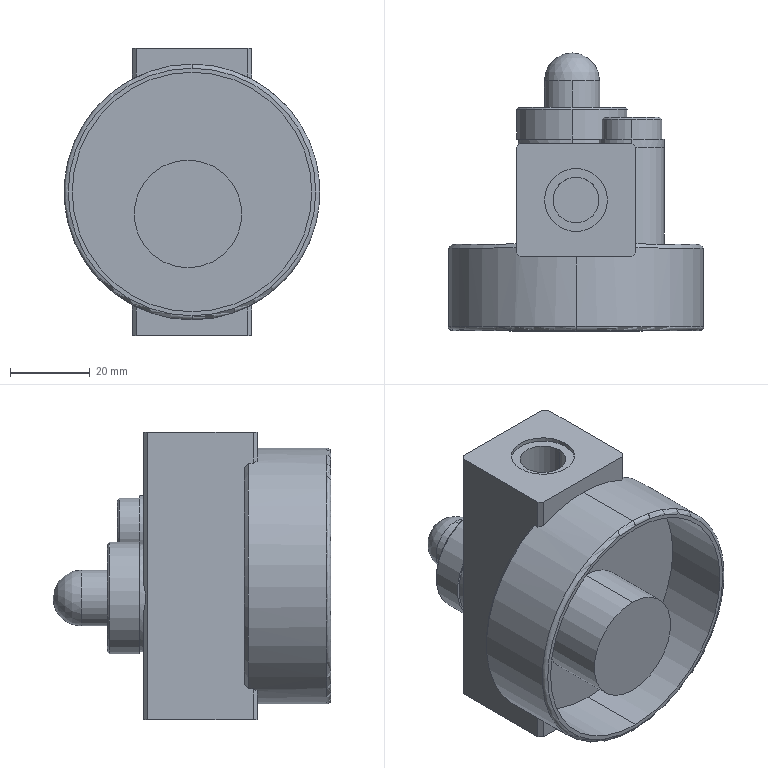Part | SolidWorks | features BaseBody 1 | 1 solid | 62 faces | box 64 x 69.6 x 72 mm | volume 94903 mm3 | plane 28 | cylinder 23 | cone 8 | torus 2 | sphere 1 | commonest cylinder face diameters 11.445 x4 15.788 x4 27 x4 14 x2 15 x2 28 x2